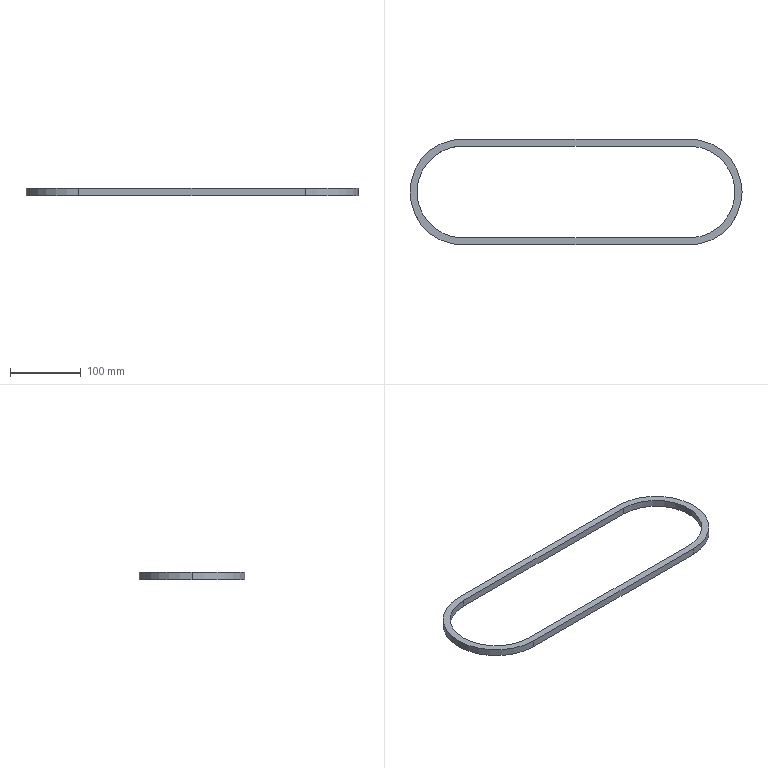Part | SolidWorks | features Extrusion 1 | 1 solid | 12 faces | box 470 x 150 x 10 mm | volume 107982 mm3 | cylinder 6 | plane 6 | commonest cylinder face diameters 130 x3 150 x3
STEP:
#1=CARTESIAN_POINT('',(0.,65.,10.));
#2=VERTEX_POINT('',#1);
#3=CARTESIAN_POINT('',(-65.,0.,10.));
#4=VERTEX_POINT('',#3);
#5=CARTESIAN_POINT('',(0.,0.,10.));
#6=DIRECTION('',(0.,0.,1.));
#7=DIRECTION('',(1.,0.,0.));
#8=AXIS2_PLACEMENT_3D('',#5,#6,#7);
#9=CIRCLE('',#8,65.);
#10=EDGE_CURVE('',#2,#4,#9,.T.);
#11=ORIENTED_EDGE('',*,*,#10,.T.);
#12=CARTESIAN_POINT('',(-65.,0.,0.));
#13=VERTEX_POINT('',#12);
#14=CARTESIAN_POINT('',(-65.,0.,10.));
#15=DIRECTION('',(0.,0.,-1.));
#16=VECTOR('',#15,1000.);
#17=LINE('',#14,#16);
#18=EDGE_CURVE('',#4,#13,#17,.T.);
#19=ORIENTED_EDGE('',*,*,#18,.T.);
#20=CARTESIAN_POINT('',(0.,65.,0.));
#21=VERTEX_POINT('',#20);
#22=CARTESIAN_POINT('',(0.,0.,0.));
#23=DIRECTION('',(0.,0.,1.));
#24=DIRECTION('',(1.,0.,0.));
#25=AXIS2_PLACEMENT_3D('',#22,#23,#24);
#26=CIRCLE('',#25,65.);
#27=EDGE_CURVE('',#21,#13,#26,.T.);
#28=ORIENTED_EDGE('',*,*,#27,.F.);
#29=CARTESIAN_POINT('',(0.,65.,10.));
#30=DIRECTION('',(0.,0.,-1.));
#31=VECTOR('',#30,1000.);
#32=LINE('',#29,#31);
#33=EDGE_CURVE('',#2,#21,#32,.T.);
#34=ORIENTED_EDGE('',*,*,#33,.F.);
#35=EDGE_LOOP('',(#11,#19,#28,#34));
#36=FACE_OUTER_BOUND('',#35,.T.);
#37=CARTESIAN_POINT('',(0.,0.,10.));
#38=DIRECTION('',(0.,0.,-1.));
#39=DIRECTION('',(-1.,0.,0.));
#40=AXIS2_PLACEMENT_3D('',#37,#38,#39);
#41=CYLINDRICAL_SURFACE('',#40,65.);
#42=ADVANCED_FACE('',(#36),#41,.F.);
#43=CARTESIAN_POINT('',(-75.,0.,10.));
#44=VERTEX_POINT('',#43);
#45=CARTESIAN_POINT('',(0.,-75.,10.));
#46=VERTEX_POINT('',#45);
#47=CARTESIAN_POINT('',(0.,0.,10.));
#48=DIRECTION('',(0.,0.,1.));
#49=DIRECTION('',(1.,0.,0.));
#50=AXIS2_PLACEMENT_3D('',#47,#48,#49);
#51=CIRCLE('',#50,75.);
#52=EDGE_CURVE('',#44,#46,#51,.T.);
#53=ORIENTED_EDGE('',*,*,#52,.F.);
#54=CARTESIAN_POINT('',(-75.,0.,0.));
#55=VERTEX_POINT('',#54);
#56=CARTESIAN_POINT('',(-75.,0.,10.));
#57=DIRECTION('',(0.,0.,-1.));
#58=VECTOR('',#57,1000.);
#59=LINE('',#56,#58);
#60=EDGE_CURVE('',#44,#55,#59,.T.);
#61=ORIENTED_EDGE('',*,*,#60,.T.);
#62=CARTESIAN_POINT('',(0.,-75.,0.));
#63=VERTEX_POINT('',#62);
#64=CARTESIAN_POINT('',(0.,0.,0.));
#65=DIRECTION('',(0.,0.,1.));
#66=DIRECTION('',(1.,0.,0.));
#67=AXIS2_PLACEMENT_3D('',#64,#65,#66);
#68=CIRCLE('',#67,75.);
#69=EDGE_CURVE('',#55,#63,#68,.T.);
#70=ORIENTED_EDGE('',*,*,#69,.T.);
#71=CARTESIAN_POINT('',(0.,-75.,10.));
#72=DIRECTION('',(0.,0.,-1.));
#73=VECTOR('',#72,1000.);
#74=LINE('',#71,#73);
#75=EDGE_CURVE('',#46,#63,#74,.T.);
#76=ORIENTED_EDGE('',*,*,#75,.F.);
#77=EDGE_LOOP('',(#53,#61,#70,#76));
#78=FACE_OUTER_BOUND('',#77,.T.);
#79=CARTESIAN_POINT('',(0.,0.,10.));
#80=DIRECTION('',(0.,0.,-1.));
#81=DIRECTION('',(-1.,0.,0.));
#82=AXIS2_PLACEMENT_3D('',#79,#80,#81);
#83=CYLINDRICAL_SURFACE('',#82,75.);
#84=ADVANCED_FACE('',(#78),#83,.T.);
#85=CARTESIAN_POINT('',(0.,75.,10.));
#86=VERTEX_POINT('',#85);
#87=CARTESIAN_POINT('',(0.,0.,10.));
#88=DIRECTION('',(0.,0.,1.));
#89=DIRECTION('',(1.,0.,0.));
#90=AXIS2_PLACEMENT_3D('',#87,#88,#89);
#91=CIRCLE('',#90,75.);
#92=EDGE_CURVE('',#86,#44,#91,.T.);
#93=ORIENTED_EDGE('',*,*,#92,.T.);
#94=ORIENTED_EDGE('',*,*,#52,.T.);
#95=CARTESIAN_POINT('',(320.,-75.,10.));
#96=VERTEX_POINT('',#95);
#97=CARTESIAN_POINT('',(0.,-75.,10.));
#98=DIRECTION('',(1.,0.,0.));
#99=VECTOR('',#98,1000.);
#100=LINE('',#97,#99);
#101=EDGE_CURVE('',#46,#96,#100,.T.);
#102=ORIENTED_EDGE('',*,*,#101,.T.);
#103=CARTESIAN_POINT('',(320.,75.,10.));
#104=VERTEX_POINT('',#103);
#105=CARTESIAN_POINT('',(320.,0.,10.));
#106=DIRECTION('',(0.,0.,1.));
#107=DIRECTION('',(1.,0.,0.));
#108=AXIS2_PLACEMENT_3D('',#105,#106,#107);
#109=CIRCLE('',#108,75.);
#110=EDGE_CURVE('',#96,#104,#109,.T.);
#111=ORIENTED_EDGE('',*,*,#110,.T.);
#112=CARTESIAN_POINT('',(0.,75.,10.));
#113=DIRECTION('',(-1.,0.,0.));
#114=VECTOR('',#113,1000.);
#115=LINE('',#112,#114);
#116=EDGE_CURVE('',#104,#86,#115,.T.);
#117=ORIENTED_EDGE('',*,*,#116,.T.);
#118=EDGE_LOOP('',(#93,#94,#102,#111,#117));
#119=FACE_OUTER_BOUND('',#118,.T.);
#120=CARTESIAN_POINT('',(0.,-65.,10.));
#121=VERTEX_POINT('',#120);
#122=CARTESIAN_POINT('',(320.,-65.,10.));
#123=VERTEX_POINT('',#122);
#124=CARTESIAN_POINT('',(0.,-65.,10.));
#125=DIRECTION('',(1.,0.,0.));
#126=VECTOR('',#125,1000.);
#127=LINE('',#124,#126);
#128=EDGE_CURVE('',#121,#123,#127,.T.);
#129=ORIENTED_EDGE('',*,*,#128,.F.);
#130=CARTESIAN_POINT('',(0.,0.,10.));
#131=DIRECTION('',(0.,0.,1.));
#132=DIRECTION('',(1.,0.,0.));
#133=AXIS2_PLACEMENT_3D('',#130,#131,#132);
#134=CIRCLE('',#133,65.);
#135=EDGE_CURVE('',#4,#121,#134,.T.);
#136=ORIENTED_EDGE('',*,*,#135,.F.);
#137=ORIENTED_EDGE('',*,*,#10,.F.);
#138=CARTESIAN_POINT('',(320.,65.,10.));
#139=VERTEX_POINT('',#138);
#140=CARTESIAN_POINT('',(0.,65.,10.));
#141=DIRECTION('',(-1.,0.,0.));
#142=VECTOR('',#141,1000.);
#143=LINE('',#140,#142);
#144=EDGE_CURVE('',#139,#2,#143,.T.);
#145=ORIENTED_EDGE('',*,*,#144,.F.);
#146=CARTESIAN_POINT('',(320.,0.,10.));
#147=DIRECTION('',(0.,0.,1.));
#148=DIRECTION('',(1.,0.,0.));
#149=AXIS2_PLACEMENT_3D('',#146,#147,#148);
#150=CIRCLE('',#149,65.);
#151=EDGE_CURVE('',#123,#139,#150,.T.);
#152=ORIENTED_EDGE('',*,*,#151,.F.);
#153=EDGE_LOOP('',(#129,#136,#137,#145,#152));
#154=FACE_BOUND('',#153,.T.);
#155=CARTESIAN_POINT('',(0.,0.,10.));
#156=DIRECTION('',(0.,0.,1.));
#157=DIRECTION('',(1.,0.,0.));
#158=AXIS2_PLACEMENT_3D('',#155,#156,#157);
#159=PLANE('',#158);
#160=ADVANCED_FACE('',(#119,#154),#159,.T.);
#161=CARTESIAN_POINT('',(0.,75.,0.));
#162=VERTEX_POINT('',#161);
#163=CARTESIAN_POINT('',(0.,0.,0.));
#164=DIRECTION('',(0.,0.,1.));
#165=DIRECTION('',(1.,0.,0.));
#166=AXIS2_PLACEMENT_3D('',#163,#164,#165);
#167=CIRCLE('',#166,75.);
#168=EDGE_CURVE('',#162,#55,#167,.T.);
#169=ORIENTED_EDGE('',*,*,#168,.F.);
#170=CARTESIAN_POINT('',(320.,75.,0.));
#171=VERTEX_POINT('',#170);
#172=CARTESIAN_POINT('',(0.,75.,0.));
#173=DIRECTION('',(-1.,0.,0.));
#174=VECTOR('',#173,1000.);
#175=LINE('',#172,#174);
#176=EDGE_CURVE('',#171,#162,#175,.T.);
#177=ORIENTED_EDGE('',*,*,#176,.F.);
#178=CARTESIAN_POINT('',(320.,-75.,0.));
#179=VERTEX_POINT('',#178);
#180=CARTESIAN_POINT('',(320.,0.,0.));
#181=DIRECTION('',(0.,0.,1.));
#182=DIRECTION('',(1.,0.,0.));
#183=AXIS2_PLACEMENT_3D('',#180,#181,#182);
#184=CIRCLE('',#183,75.);
#185=EDGE_CURVE('',#179,#171,#184,.T.);
#186=ORIENTED_EDGE('',*,*,#185,.F.);
#187=CARTESIAN_POINT('',(0.,-75.,0.));
#188=DIRECTION('',(1.,0.,0.));
#189=VECTOR('',#188,1000.);
#190=LINE('',#187,#189);
#191=EDGE_CURVE('',#63,#179,#190,.T.);
#192=ORIENTED_EDGE('',*,*,#191,.F.);
#193=ORIENTED_EDGE('',*,*,#69,.F.);
#194=EDGE_LOOP('',(#169,#177,#186,#192,#193));
#195=FACE_OUTER_BOUND('',#194,.T.);
#196=ORIENTED_EDGE('',*,*,#27,.T.);
#197=CARTESIAN_POINT('',(0.,-65.,0.));
#198=VERTEX_POINT('',#197);
#199=CARTESIAN_POINT('',(0.,0.,0.));
#200=DIRECTION('',(0.,0.,1.));
#201=DIRECTION('',(1.,0.,0.));
#202=AXIS2_PLACEMENT_3D('',#199,#200,#201);
#203=CIRCLE('',#202,65.);
#204=EDGE_CURVE('',#13,#198,#203,.T.);
#205=ORIENTED_EDGE('',*,*,#204,.T.);
#206=CARTESIAN_POINT('',(320.,-65.,0.));
#207=VERTEX_POINT('',#206);
#208=CARTESIAN_POINT('',(0.,-65.,0.));
#209=DIRECTION('',(1.,0.,0.));
#210=VECTOR('',#209,1000.);
#211=LINE('',#208,#210);
#212=EDGE_CURVE('',#198,#207,#211,.T.);
#213=ORIENTED_EDGE('',*,*,#212,.T.);
#214=CARTESIAN_POINT('',(320.,65.,0.));
#215=VERTEX_POINT('',#214);
#216=CARTESIAN_POINT('',(320.,0.,0.));
#217=DIRECTION('',(0.,0.,1.));
#218=DIRECTION('',(1.,0.,0.));
#219=AXIS2_PLACEMENT_3D('',#216,#217,#218);
#220=CIRCLE('',#219,65.);
#221=EDGE_CURVE('',#207,#215,#220,.T.);
#222=ORIENTED_EDGE('',*,*,#221,.T.);
#223=CARTESIAN_POINT('',(0.,65.,0.));
#224=DIRECTION('',(-1.,0.,0.));
#225=VECTOR('',#224,1000.);
#226=LINE('',#223,#225);
#227=EDGE_CURVE('',#215,#21,#226,.T.);
#228=ORIENTED_EDGE('',*,*,#227,.T.);
#229=EDGE_LOOP('',(#196,#205,#213,#222,#228));
#230=FACE_BOUND('',#229,.T.);
#231=CARTESIAN_POINT('',(0.,0.,0.));
#232=DIRECTION('',(0.,0.,1.));
#233=DIRECTION('',(1.,0.,0.));
#234=AXIS2_PLACEMENT_3D('',#231,#232,#233);
#235=PLANE('',#234);
#236=ADVANCED_FACE('',(#195,#230),#235,.F.);
#237=ORIENTED_EDGE('',*,*,#60,.F.);
#238=ORIENTED_EDGE('',*,*,#92,.F.);
#239=CARTESIAN_POINT('',(0.,75.,10.));
#240=DIRECTION('',(0.,0.,-1.));
#241=VECTOR('',#240,1000.);
#242=LINE('',#239,#241);
#243=EDGE_CURVE('',#86,#162,#242,.T.);
#244=ORIENTED_EDGE('',*,*,#243,.T.);
#245=ORIENTED_EDGE('',*,*,#168,.T.);
#246=EDGE_LOOP('',(#237,#238,#244,#245));
#247=FACE_OUTER_BOUND('',#246,.T.);
#248=CARTESIAN_POINT('',(0.,0.,10.));
#249=DIRECTION('',(0.,0.,-1.));
#250=DIRECTION('',(-1.,0.,0.));
#251=AXIS2_PLACEMENT_3D('',#248,#249,#250);
#252=CYLINDRICAL_SURFACE('',#251,75.);
#253=ADVANCED_FACE('',(#247),#252,.T.);
#254=ORIENTED_EDGE('',*,*,#191,.T.);
#255=CARTESIAN_POINT('',(320.,-75.,10.));
#256=DIRECTION('',(0.,0.,-1.));
#257=VECTOR('',#256,1000.);
#258=LINE('',#255,#257);
#259=EDGE_CURVE('',#96,#179,#258,.T.);
#260=ORIENTED_EDGE('',*,*,#259,.F.);
#261=ORIENTED_EDGE('',*,*,#101,.F.);
#262=ORIENTED_EDGE('',*,*,#75,.T.);
#263=EDGE_LOOP('',(#254,#260,#261,#262));
#264=FACE_OUTER_BOUND('',#263,.T.);
#265=CARTESIAN_POINT('',(0.,-75.,10.));
#266=DIRECTION('',(0.,1.,0.));
#267=DIRECTION('',(0.,0.,1.));
#268=AXIS2_PLACEMENT_3D('',#265,#266,#267);
#269=PLANE('',#268);
#270=ADVANCED_FACE('',(#264),#269,.F.);
#271=ORIENTED_EDGE('',*,*,#185,.T.);
#272=CARTESIAN_POINT('',(320.,75.,10.));
#273=DIRECTION('',(0.,0.,-1.));
#274=VECTOR('',#273,1000.);
#275=LINE('',#272,#274);
#276=EDGE_CURVE('',#104,#171,#275,.T.);
#277=ORIENTED_EDGE('',*,*,#276,.F.);
#278=ORIENTED_EDGE('',*,*,#110,.F.);
#279=ORIENTED_EDGE('',*,*,#259,.T.);
#280=EDGE_LOOP('',(#271,#277,#278,#279));
#281=FACE_OUTER_BOUND('',#280,.T.);
#282=CARTESIAN_POINT('',(320.,0.,10.));
#283=DIRECTION('',(0.,0.,-1.));
#284=DIRECTION('',(-1.,0.,0.));
#285=AXIS2_PLACEMENT_3D('',#282,#283,#284);
#286=CYLINDRICAL_SURFACE('',#285,75.);
#287=ADVANCED_FACE('',(#281),#286,.T.);
#288=ORIENTED_EDGE('',*,*,#176,.T.);
#289=ORIENTED_EDGE('',*,*,#243,.F.);
#290=ORIENTED_EDGE('',*,*,#116,.F.);
#291=ORIENTED_EDGE('',*,*,#276,.T.);
#292=EDGE_LOOP('',(#288,#289,#290,#291));
#293=FACE_OUTER_BOUND('',#292,.T.);
#294=CARTESIAN_POINT('',(0.,75.,10.));
#295=DIRECTION('',(0.,-1.,0.));
#296=DIRECTION('',(0.,0.,-1.));
#297=AXIS2_PLACEMENT_3D('',#294,#295,#296);
#298=PLANE('',#297);
#299=ADVANCED_FACE('',(#293),#298,.F.);
#300=ORIENTED_EDGE('',*,*,#18,.F.);
#301=ORIENTED_EDGE('',*,*,#135,.T.);
#302=CARTESIAN_POINT('',(0.,-65.,10.));
#303=DIRECTION('',(0.,0.,-1.));
#304=VECTOR('',#303,1000.);
#305=LINE('',#302,#304);
#306=EDGE_CURVE('',#121,#198,#305,.T.);
#307=ORIENTED_EDGE('',*,*,#306,.T.);
#308=ORIENTED_EDGE('',*,*,#204,.F.);
#309=EDGE_LOOP('',(#300,#301,#307,#308));
#310=FACE_OUTER_BOUND('',#309,.T.);
#311=CARTESIAN_POINT('',(0.,0.,10.));
#312=DIRECTION('',(0.,0.,-1.));
#313=DIRECTION('',(-1.,0.,0.));
#314=AXIS2_PLACEMENT_3D('',#311,#312,#313);
#315=CYLINDRICAL_SURFACE('',#314,65.);
#316=ADVANCED_FACE('',(#310),#315,.F.);
#317=ORIENTED_EDGE('',*,*,#212,.F.);
#318=ORIENTED_EDGE('',*,*,#306,.F.);
#319=ORIENTED_EDGE('',*,*,#128,.T.);
#320=CARTESIAN_POINT('',(320.,-65.,10.));
#321=DIRECTION('',(0.,0.,-1.));
#322=VECTOR('',#321,1000.);
#323=LINE('',#320,#322);
#324=EDGE_CURVE('',#123,#207,#323,.T.);
#325=ORIENTED_EDGE('',*,*,#324,.T.);
#326=EDGE_LOOP('',(#317,#318,#319,#325));
#327=FACE_OUTER_BOUND('',#326,.T.);
#328=CARTESIAN_POINT('',(0.,-65.,10.));
#329=DIRECTION('',(0.,1.,0.));
#330=DIRECTION('',(0.,0.,1.));
#331=AXIS2_PLACEMENT_3D('',#328,#329,#330);
#332=PLANE('',#331);
#333=ADVANCED_FACE('',(#327),#332,.T.);
#334=ORIENTED_EDGE('',*,*,#221,.F.);
#335=ORIENTED_EDGE('',*,*,#324,.F.);
#336=ORIENTED_EDGE('',*,*,#151,.T.);
#337=CARTESIAN_POINT('',(320.,65.,10.));
#338=DIRECTION('',(0.,0.,-1.));
#339=VECTOR('',#338,1000.);
#340=LINE('',#337,#339);
#341=EDGE_CURVE('',#139,#215,#340,.T.);
#342=ORIENTED_EDGE('',*,*,#341,.T.);
#343=EDGE_LOOP('',(#334,#335,#336,#342));
#344=FACE_OUTER_BOUND('',#343,.T.);
#345=CARTESIAN_POINT('',(320.,0.,10.));
#346=DIRECTION('',(0.,0.,-1.));
#347=DIRECTION('',(-1.,0.,0.));
#348=AXIS2_PLACEMENT_3D('',#345,#346,#347);
#349=CYLINDRICAL_SURFACE('',#348,65.);
#350=ADVANCED_FACE('',(#344),#349,.F.);
#351=ORIENTED_EDGE('',*,*,#227,.F.);
#352=ORIENTED_EDGE('',*,*,#341,.F.);
#353=ORIENTED_EDGE('',*,*,#144,.T.);
#354=ORIENTED_EDGE('',*,*,#33,.T.);
#355=EDGE_LOOP('',(#351,#352,#353,#354));
#356=FACE_OUTER_BOUND('',#355,.T.);
#357=CARTESIAN_POINT('',(0.,65.,10.));
#358=DIRECTION('',(0.,-1.,0.));
#359=DIRECTION('',(0.,0.,-1.));
#360=AXIS2_PLACEMENT_3D('',#357,#358,#359);
#361=PLANE('',#360);
#362=ADVANCED_FACE('',(#356),#361,.T.);
#363=CLOSED_SHELL('',(#42,#84,#160,#236,#253,#270,#287,#299,#316,#333,#350,#362));
#364=MANIFOLD_SOLID_BREP('',#363);
#365=CARTESIAN_POINT('',(0.,0.,0.));
#366=DIRECTION('',(0.,0.,1.));
#367=DIRECTION('',(1.,0.,0.));
#368=AXIS2_PLACEMENT_3D('',#365,#366,#367);
#369=(LENGTH_UNIT()NAMED_UNIT(*)SI_UNIT(.MILLI.,.METRE.));
#370=UNCERTAINTY_MEASURE_WITH_UNIT(LENGTH_MEASURE(0.00001),#369,'','');
#371=(NAMED_UNIT(*)PLANE_ANGLE_UNIT()SI_UNIT($,.RADIAN.));
#372=(NAMED_UNIT(*)SI_UNIT($,.STERADIAN.)SOLID_ANGLE_UNIT());
#373=(GEOMETRIC_REPRESENTATION_CONTEXT(3)GLOBAL_UNCERTAINTY_ASSIGNED_CONTEXT((#370))GLOBAL_UNIT_ASSIGNED_CONTEXT((#369,#371,#372))REPRESENTATION_CONTEXT('',''));
#374=ADVANCED_BREP_SHAPE_REPRESENTATION('',(#364,#368),#373);